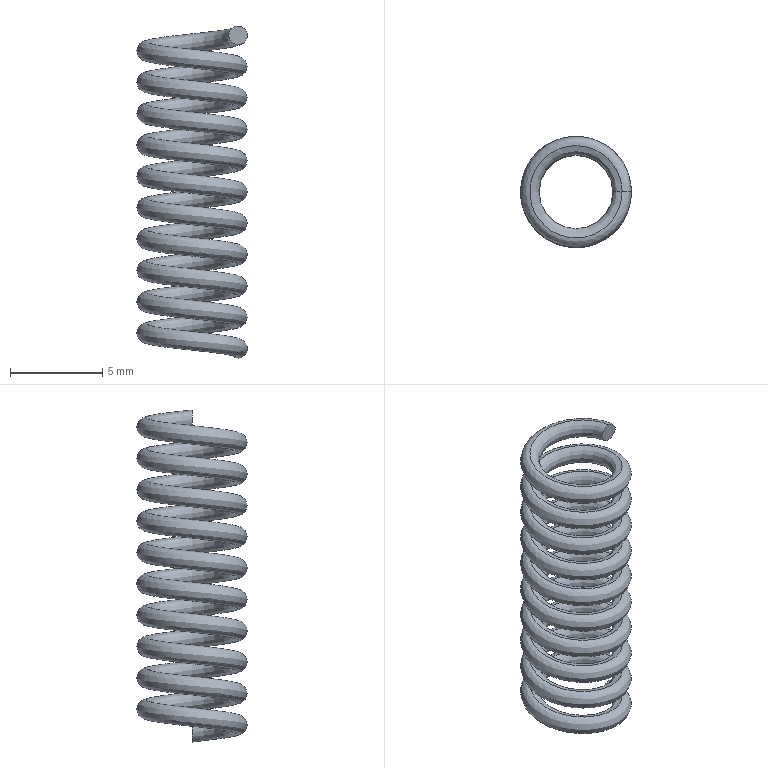Part | SolidWorks | features Helix 1, Sweep 1 | 1 solid | 4 faces | box 6 x 6 x 18 mm | volume 123.415 mm3 | spline 2 | plane 2